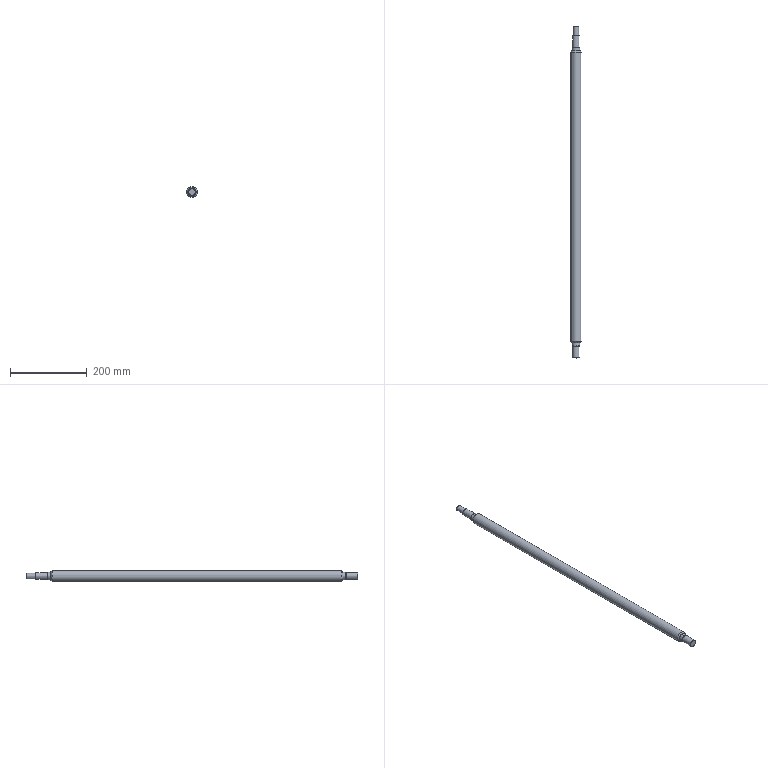Part | NX | features CHAMFER 2, DATUM_CSYS 2, SKETCH 1, SWP104 1, SYMBOLIC_THREAD 1, TRIM BODY 1 | 1 solid | 20 faces | box 28 x 865 x 28 mm | volume 492482 mm3 | plane 7 | cone 7 | cylinder 6 | commonest cylinder face diameters 18 x2 20 x2 14 x1 28 x1
STEP:
#1=CARTESIAN_POINT('',(0.,865.,6.5));
#2=VERTEX_POINT('',#1);
#3=CARTESIAN_POINT('',(0.,865.,0.));
#4=DIRECTION('',(0.,1.,0.));
#5=DIRECTION('',(0.,0.,1.));
#6=AXIS2_PLACEMENT_3D('',#3,#4,#5);
#7=CIRCLE('',#6,6.5);
#8=EDGE_CURVE('',#2,#2,#7,.T.);
#9=ORIENTED_EDGE('',*,*,#8,.T.);
#10=EDGE_LOOP('',(#9));
#11=FACE_BOUND('',#10,.T.);
#12=CARTESIAN_POINT('',(0.,865.,0.));
#13=DIRECTION('',(0.,1.,0.));
#14=DIRECTION('',(0.,0.,1.));
#15=AXIS2_PLACEMENT_3D('',#12,#13,#14);
#16=PLANE('',#15);
#17=ADVANCED_FACE('',(#11),#16,.T.);
#18=CARTESIAN_POINT('',(0.,864.5,7.));
#19=VERTEX_POINT('',#18);
#20=CARTESIAN_POINT('',(0.,864.5,0.));
#21=DIRECTION('',(0.,1.,0.));
#22=DIRECTION('',(0.,0.,1.));
#23=AXIS2_PLACEMENT_3D('',#20,#21,#22);
#24=CIRCLE('',#23,7.);
#25=EDGE_CURVE('',#19,#19,#24,.F.);
#26=ORIENTED_EDGE('',*,*,#25,.T.);
#27=EDGE_LOOP('',(#26));
#28=FACE_BOUND('',#27,.T.);
#29=CARTESIAN_POINT('',(0.,840.,7.));
#30=VERTEX_POINT('',#29);
#31=CARTESIAN_POINT('',(0.,840.,0.));
#32=DIRECTION('',(0.,1.,0.));
#33=DIRECTION('',(0.,0.,1.));
#34=AXIS2_PLACEMENT_3D('',#31,#32,#33);
#35=CIRCLE('',#34,7.);
#36=EDGE_CURVE('',#30,#30,#35,.T.);
#37=ORIENTED_EDGE('',*,*,#36,.T.);
#38=EDGE_LOOP('',(#37));
#39=FACE_BOUND('',#38,.T.);
#40=CARTESIAN_POINT('',(0.,0.,0.));
#41=DIRECTION('',(0.,1.,0.));
#42=DIRECTION('',(0.,0.,1.));
#43=AXIS2_PLACEMENT_3D('',#40,#41,#42);
#44=CYLINDRICAL_SURFACE('',#43,7.);
#45=ADVANCED_FACE('',(#28,#39),#44,.T.);
#46=CARTESIAN_POINT('',(0.,840.,-8.5));
#47=VERTEX_POINT('',#46);
#48=CARTESIAN_POINT('',(0.,840.,0.));
#49=DIRECTION('',(0.,-1.,0.));
#50=DIRECTION('',(0.,0.,-1.));
#51=AXIS2_PLACEMENT_3D('',#48,#49,#50);
#52=CIRCLE('',#51,8.5);
#53=EDGE_CURVE('',#47,#47,#52,.F.);
#54=ORIENTED_EDGE('',*,*,#53,.T.);
#55=EDGE_LOOP('',(#54));
#56=FACE_BOUND('',#55,.T.);
#57=ORIENTED_EDGE('',*,*,#36,.F.);
#58=EDGE_LOOP('',(#57));
#59=FACE_BOUND('',#58,.T.);
#60=CARTESIAN_POINT('',(0.,840.,9.));
#61=DIRECTION('',(0.,-1.,0.));
#62=DIRECTION('',(0.,0.,-1.));
#63=AXIS2_PLACEMENT_3D('',#60,#61,#62);
#64=PLANE('',#63);
#65=ADVANCED_FACE('',(#56,#59),#64,.F.);
#66=CARTESIAN_POINT('',(0.,839.5,-9.));
#67=VERTEX_POINT('',#66);
#68=CARTESIAN_POINT('',(0.,839.5,0.));
#69=DIRECTION('',(0.,-1.,0.));
#70=DIRECTION('',(0.,0.,-1.));
#71=AXIS2_PLACEMENT_3D('',#68,#69,#70);
#72=CIRCLE('',#71,9.);
#73=EDGE_CURVE('',#67,#67,#72,.T.);
#74=ORIENTED_EDGE('',*,*,#73,.T.);
#75=EDGE_LOOP('',(#74));
#76=FACE_BOUND('',#75,.T.);
#77=CARTESIAN_POINT('',(0.,809.,9.));
#78=VERTEX_POINT('',#77);
#79=CARTESIAN_POINT('',(0.,809.,0.));
#80=DIRECTION('',(0.,1.,0.));
#81=DIRECTION('',(0.,0.,1.));
#82=AXIS2_PLACEMENT_3D('',#79,#80,#81);
#83=CIRCLE('',#82,9.);
#84=EDGE_CURVE('',#78,#78,#83,.T.);
#85=ORIENTED_EDGE('',*,*,#84,.T.);
#86=EDGE_LOOP('',(#85));
#87=FACE_BOUND('',#86,.T.);
#88=CARTESIAN_POINT('',(0.,0.,0.));
#89=DIRECTION('',(0.,1.,0.));
#90=DIRECTION('',(0.,0.,1.));
#91=AXIS2_PLACEMENT_3D('',#88,#89,#90);
#92=CYLINDRICAL_SURFACE('',#91,9.);
#93=ADVANCED_FACE('',(#76,#87),#92,.T.);
#94=CARTESIAN_POINT('',(0.,809.,-9.5));
#95=VERTEX_POINT('',#94);
#96=CARTESIAN_POINT('',(0.,809.,0.));
#97=DIRECTION('',(0.,-1.,0.));
#98=DIRECTION('',(0.,0.,-1.));
#99=AXIS2_PLACEMENT_3D('',#96,#97,#98);
#100=CIRCLE('',#99,9.5);
#101=EDGE_CURVE('',#95,#95,#100,.F.);
#102=ORIENTED_EDGE('',*,*,#101,.T.);
#103=EDGE_LOOP('',(#102));
#104=FACE_BOUND('',#103,.T.);
#105=ORIENTED_EDGE('',*,*,#84,.F.);
#106=EDGE_LOOP('',(#105));
#107=FACE_BOUND('',#106,.T.);
#108=CARTESIAN_POINT('',(0.,809.,10.));
#109=DIRECTION('',(0.,-1.,0.));
#110=DIRECTION('',(0.,0.,-1.));
#111=AXIS2_PLACEMENT_3D('',#108,#109,#110);
#112=PLANE('',#111);
#113=ADVANCED_FACE('',(#104,#107),#112,.F.);
#114=CARTESIAN_POINT('',(0.,808.5,-10.));
#115=VERTEX_POINT('',#114);
#116=CARTESIAN_POINT('',(0.,808.5,0.));
#117=DIRECTION('',(0.,-1.,0.));
#118=DIRECTION('',(0.,0.,-1.));
#119=AXIS2_PLACEMENT_3D('',#116,#117,#118);
#120=CIRCLE('',#119,10.);
#121=EDGE_CURVE('',#115,#115,#120,.T.);
#122=ORIENTED_EDGE('',*,*,#121,.T.);
#123=EDGE_LOOP('',(#122));
#124=FACE_BOUND('',#123,.T.);
#125=CARTESIAN_POINT('',(0.,800.,10.));
#126=VERTEX_POINT('',#125);
#127=CARTESIAN_POINT('',(0.,800.,0.));
#128=DIRECTION('',(0.,1.,0.));
#129=DIRECTION('',(0.,0.,1.));
#130=AXIS2_PLACEMENT_3D('',#127,#128,#129);
#131=CIRCLE('',#130,10.);
#132=EDGE_CURVE('',#126,#126,#131,.T.);
#133=ORIENTED_EDGE('',*,*,#132,.T.);
#134=EDGE_LOOP('',(#133));
#135=FACE_BOUND('',#134,.T.);
#136=CARTESIAN_POINT('',(0.,0.,0.));
#137=DIRECTION('',(0.,1.,0.));
#138=DIRECTION('',(0.,0.,1.));
#139=AXIS2_PLACEMENT_3D('',#136,#137,#138);
#140=CYLINDRICAL_SURFACE('',#139,10.);
#141=ADVANCED_FACE('',(#124,#135),#140,.T.);
#142=CARTESIAN_POINT('',(0.,800.,-11.));
#143=VERTEX_POINT('',#142);
#144=CARTESIAN_POINT('',(0.,800.,0.));
#145=DIRECTION('',(0.,-1.,0.));
#146=DIRECTION('',(0.,0.,-1.));
#147=AXIS2_PLACEMENT_3D('',#144,#145,#146);
#148=CIRCLE('',#147,11.);
#149=EDGE_CURVE('',#143,#143,#148,.F.);
#150=ORIENTED_EDGE('',*,*,#149,.T.);
#151=EDGE_LOOP('',(#150));
#152=FACE_BOUND('',#151,.T.);
#153=ORIENTED_EDGE('',*,*,#132,.F.);
#154=EDGE_LOOP('',(#153));
#155=FACE_BOUND('',#154,.T.);
#156=CARTESIAN_POINT('',(0.,800.,14.));
#157=DIRECTION('',(0.,-1.,0.));
#158=DIRECTION('',(0.,0.,-1.));
#159=AXIS2_PLACEMENT_3D('',#156,#157,#158);
#160=PLANE('',#159);
#161=ADVANCED_FACE('',(#152,#155),#160,.F.);
#162=CARTESIAN_POINT('',(0.,43.,14.));
#163=VERTEX_POINT('',#162);
#164=CARTESIAN_POINT('',(0.,43.,0.));
#165=DIRECTION('',(0.,1.,0.));
#166=DIRECTION('',(0.,0.,1.));
#167=AXIS2_PLACEMENT_3D('',#164,#165,#166);
#168=CIRCLE('',#167,14.);
#169=EDGE_CURVE('',#163,#163,#168,.T.);
#170=ORIENTED_EDGE('',*,*,#169,.T.);
#171=EDGE_LOOP('',(#170));
#172=FACE_BOUND('',#171,.T.);
#173=CARTESIAN_POINT('',(0.,797.,-14.));
#174=VERTEX_POINT('',#173);
#175=CARTESIAN_POINT('',(0.,797.,0.));
#176=DIRECTION('',(0.,-1.,0.));
#177=DIRECTION('',(0.,0.,-1.));
#178=AXIS2_PLACEMENT_3D('',#175,#176,#177);
#179=CIRCLE('',#178,14.);
#180=EDGE_CURVE('',#174,#174,#179,.T.);
#181=ORIENTED_EDGE('',*,*,#180,.T.);
#182=EDGE_LOOP('',(#181));
#183=FACE_BOUND('',#182,.T.);
#184=CARTESIAN_POINT('',(0.,0.,0.));
#185=DIRECTION('',(0.,1.,0.));
#186=DIRECTION('',(0.,0.,1.));
#187=AXIS2_PLACEMENT_3D('',#184,#185,#186);
#188=CYLINDRICAL_SURFACE('',#187,14.);
#189=ADVANCED_FACE('',(#172,#183),#188,.T.);
#190=CARTESIAN_POINT('',(0.,40.,11.));
#191=VERTEX_POINT('',#190);
#192=CARTESIAN_POINT('',(0.,40.,0.));
#193=DIRECTION('',(0.,1.,0.));
#194=DIRECTION('',(0.,0.,1.));
#195=AXIS2_PLACEMENT_3D('',#192,#193,#194);
#196=CIRCLE('',#195,11.);
#197=EDGE_CURVE('',#191,#191,#196,.F.);
#198=ORIENTED_EDGE('',*,*,#197,.T.);
#199=EDGE_LOOP('',(#198));
#200=FACE_BOUND('',#199,.T.);
#201=CARTESIAN_POINT('',(0.,40.,10.));
#202=VERTEX_POINT('',#201);
#203=CARTESIAN_POINT('',(0.,40.,0.));
#204=DIRECTION('',(0.,1.,0.));
#205=DIRECTION('',(0.,0.,1.));
#206=AXIS2_PLACEMENT_3D('',#203,#204,#205);
#207=CIRCLE('',#206,10.);
#208=EDGE_CURVE('',#202,#202,#207,.T.);
#209=ORIENTED_EDGE('',*,*,#208,.T.);
#210=EDGE_LOOP('',(#209));
#211=FACE_BOUND('',#210,.T.);
#212=CARTESIAN_POINT('',(0.,40.,10.));
#213=DIRECTION('',(0.,1.,0.));
#214=DIRECTION('',(0.,0.,1.));
#215=AXIS2_PLACEMENT_3D('',#212,#213,#214);
#216=PLANE('',#215);
#217=ADVANCED_FACE('',(#200,#211),#216,.F.);
#218=CARTESIAN_POINT('',(0.,31.5,10.));
#219=VERTEX_POINT('',#218);
#220=CARTESIAN_POINT('',(0.,31.5,0.));
#221=DIRECTION('',(0.,1.,0.));
#222=DIRECTION('',(0.,0.,1.));
#223=AXIS2_PLACEMENT_3D('',#220,#221,#222);
#224=CIRCLE('',#223,10.);
#225=EDGE_CURVE('',#219,#219,#224,.T.);
#226=ORIENTED_EDGE('',*,*,#225,.T.);
#227=EDGE_LOOP('',(#226));
#228=FACE_BOUND('',#227,.T.);
#229=ORIENTED_EDGE('',*,*,#208,.F.);
#230=EDGE_LOOP('',(#229));
#231=FACE_BOUND('',#230,.T.);
#232=CARTESIAN_POINT('',(0.,0.,0.));
#233=DIRECTION('',(0.,1.,0.));
#234=DIRECTION('',(0.,0.,1.));
#235=AXIS2_PLACEMENT_3D('',#232,#233,#234);
#236=CYLINDRICAL_SURFACE('',#235,10.);
#237=ADVANCED_FACE('',(#228,#231),#236,.T.);
#238=CARTESIAN_POINT('',(0.,31.,9.5));
#239=VERTEX_POINT('',#238);
#240=CARTESIAN_POINT('',(0.,31.,0.));
#241=DIRECTION('',(0.,1.,0.));
#242=DIRECTION('',(0.,0.,1.));
#243=AXIS2_PLACEMENT_3D('',#240,#241,#242);
#244=CIRCLE('',#243,9.5);
#245=EDGE_CURVE('',#239,#239,#244,.F.);
#246=ORIENTED_EDGE('',*,*,#245,.T.);
#247=EDGE_LOOP('',(#246));
#248=FACE_BOUND('',#247,.T.);
#249=CARTESIAN_POINT('',(0.,31.,9.));
#250=VERTEX_POINT('',#249);
#251=CARTESIAN_POINT('',(0.,31.,0.));
#252=DIRECTION('',(0.,1.,0.));
#253=DIRECTION('',(0.,0.,1.));
#254=AXIS2_PLACEMENT_3D('',#251,#252,#253);
#255=CIRCLE('',#254,9.);
#256=EDGE_CURVE('',#250,#250,#255,.T.);
#257=ORIENTED_EDGE('',*,*,#256,.T.);
#258=EDGE_LOOP('',(#257));
#259=FACE_BOUND('',#258,.T.);
#260=CARTESIAN_POINT('',(0.,31.,9.));
#261=DIRECTION('',(0.,1.,0.));
#262=DIRECTION('',(0.,0.,1.));
#263=AXIS2_PLACEMENT_3D('',#260,#261,#262);
#264=PLANE('',#263);
#265=ADVANCED_FACE('',(#248,#259),#264,.F.);
#266=CARTESIAN_POINT('',(0.,0.5,9.));
#267=VERTEX_POINT('',#266);
#268=CARTESIAN_POINT('',(0.,0.5,0.));
#269=DIRECTION('',(0.,1.,0.));
#270=DIRECTION('',(0.,0.,1.));
#271=AXIS2_PLACEMENT_3D('',#268,#269,#270);
#272=CIRCLE('',#271,9.);
#273=EDGE_CURVE('',#267,#267,#272,.T.);
#274=ORIENTED_EDGE('',*,*,#273,.T.);
#275=EDGE_LOOP('',(#274));
#276=FACE_BOUND('',#275,.T.);
#277=ORIENTED_EDGE('',*,*,#256,.F.);
#278=EDGE_LOOP('',(#277));
#279=FACE_BOUND('',#278,.T.);
#280=CARTESIAN_POINT('',(0.,0.,0.));
#281=DIRECTION('',(0.,1.,0.));
#282=DIRECTION('',(0.,0.,1.));
#283=AXIS2_PLACEMENT_3D('',#280,#281,#282);
#284=CYLINDRICAL_SURFACE('',#283,9.);
#285=ADVANCED_FACE('',(#276,#279),#284,.T.);
#286=CARTESIAN_POINT('',(0.,0.,8.5));
#287=VERTEX_POINT('',#286);
#288=CARTESIAN_POINT('',(0.,0.,0.));
#289=DIRECTION('',(0.,1.,0.));
#290=DIRECTION('',(0.,0.,1.));
#291=AXIS2_PLACEMENT_3D('',#288,#289,#290);
#292=CIRCLE('',#291,8.5);
#293=EDGE_CURVE('',#287,#287,#292,.F.);
#294=ORIENTED_EDGE('',*,*,#293,.T.);
#295=EDGE_LOOP('',(#294));
#296=FACE_BOUND('',#295,.T.);
#297=CARTESIAN_POINT('',(0.,0.,7.));
#298=DIRECTION('',(0.,1.,0.));
#299=DIRECTION('',(0.,0.,1.));
#300=AXIS2_PLACEMENT_3D('',#297,#298,#299);
#301=PLANE('',#300);
#302=ADVANCED_FACE('',(#296),#301,.F.);
#303=ORIENTED_EDGE('',*,*,#197,.F.);
#304=EDGE_LOOP('',(#303));
#305=FACE_BOUND('',#304,.T.);
#306=ORIENTED_EDGE('',*,*,#169,.F.);
#307=EDGE_LOOP('',(#306));
#308=FACE_BOUND('',#307,.T.);
#309=CARTESIAN_POINT('',(0.,43.,0.));
#310=DIRECTION('',(0.,1.,0.));
#311=DIRECTION('',(0.,0.,1.));
#312=AXIS2_PLACEMENT_3D('',#309,#310,#311);
#313=CONICAL_SURFACE('',#312,14.,0.7854);
#314=ADVANCED_FACE('',(#305,#308),#313,.T.);
#315=ORIENTED_EDGE('',*,*,#180,.F.);
#316=EDGE_LOOP('',(#315));
#317=FACE_BOUND('',#316,.T.);
#318=ORIENTED_EDGE('',*,*,#149,.F.);
#319=EDGE_LOOP('',(#318));
#320=FACE_BOUND('',#319,.T.);
#321=CARTESIAN_POINT('',(0.,800.,0.));
#322=DIRECTION('',(0.,-1.,0.));
#323=DIRECTION('',(0.,0.,-1.));
#324=AXIS2_PLACEMENT_3D('',#321,#322,#323);
#325=CONICAL_SURFACE('',#324,11.,0.7854);
#326=ADVANCED_FACE('',(#317,#320),#325,.T.);
#327=ORIENTED_EDGE('',*,*,#73,.F.);
#328=EDGE_LOOP('',(#327));
#329=FACE_BOUND('',#328,.T.);
#330=ORIENTED_EDGE('',*,*,#53,.F.);
#331=EDGE_LOOP('',(#330));
#332=FACE_BOUND('',#331,.T.);
#333=CARTESIAN_POINT('',(0.,840.,0.));
#334=DIRECTION('',(0.,-1.,0.));
#335=DIRECTION('',(0.,0.,-1.));
#336=AXIS2_PLACEMENT_3D('',#333,#334,#335);
#337=CONICAL_SURFACE('',#336,8.5,0.7854);
#338=ADVANCED_FACE('',(#329,#332),#337,.T.);
#339=ORIENTED_EDGE('',*,*,#121,.F.);
#340=EDGE_LOOP('',(#339));
#341=FACE_BOUND('',#340,.T.);
#342=ORIENTED_EDGE('',*,*,#101,.F.);
#343=EDGE_LOOP('',(#342));
#344=FACE_BOUND('',#343,.T.);
#345=CARTESIAN_POINT('',(0.,809.,0.));
#346=DIRECTION('',(0.,-1.,0.));
#347=DIRECTION('',(0.,0.,-1.));
#348=AXIS2_PLACEMENT_3D('',#345,#346,#347);
#349=CONICAL_SURFACE('',#348,9.5,0.7854);
#350=ADVANCED_FACE('',(#341,#344),#349,.T.);
#351=ORIENTED_EDGE('',*,*,#25,.F.);
#352=EDGE_LOOP('',(#351));
#353=FACE_BOUND('',#352,.T.);
#354=ORIENTED_EDGE('',*,*,#8,.F.);
#355=EDGE_LOOP('',(#354));
#356=FACE_BOUND('',#355,.T.);
#357=CARTESIAN_POINT('',(0.,865.,0.));
#358=DIRECTION('',(0.,-1.,0.));
#359=DIRECTION('',(0.,0.,-1.));
#360=AXIS2_PLACEMENT_3D('',#357,#358,#359);
#361=CONICAL_SURFACE('',#360,6.5,0.7854);
#362=ADVANCED_FACE('',(#353,#356),#361,.T.);
#363=ORIENTED_EDGE('',*,*,#293,.F.);
#364=EDGE_LOOP('',(#363));
#365=FACE_BOUND('',#364,.T.);
#366=ORIENTED_EDGE('',*,*,#273,.F.);
#367=EDGE_LOOP('',(#366));
#368=FACE_BOUND('',#367,.T.);
#369=CARTESIAN_POINT('',(0.,0.5,0.));
#370=DIRECTION('',(0.,1.,0.));
#371=DIRECTION('',(0.,0.,1.));
#372=AXIS2_PLACEMENT_3D('',#369,#370,#371);
#373=CONICAL_SURFACE('',#372,9.,0.7854);
#374=ADVANCED_FACE('',(#365,#368),#373,.T.);
#375=ORIENTED_EDGE('',*,*,#245,.F.);
#376=EDGE_LOOP('',(#375));
#377=FACE_BOUND('',#376,.T.);
#378=ORIENTED_EDGE('',*,*,#225,.F.);
#379=EDGE_LOOP('',(#378));
#380=FACE_BOUND('',#379,.T.);
#381=CARTESIAN_POINT('',(0.,31.5,0.));
#382=DIRECTION('',(0.,1.,0.));
#383=DIRECTION('',(0.,0.,1.));
#384=AXIS2_PLACEMENT_3D('',#381,#382,#383);
#385=CONICAL_SURFACE('',#384,10.,0.7854);
#386=ADVANCED_FACE('',(#377,#380),#385,.T.);
#387=CLOSED_SHELL('',(#17,#45,#65,#93,#113,#141,#161,#189,#217,#237,#265,#285,#302,#314,#326,#338,#350,#362,#374,#386));
#388=MANIFOLD_SOLID_BREP('',#387);
#389=(LENGTH_UNIT()NAMED_UNIT(*)SI_UNIT(.MILLI.,.METRE.));
#390=UNCERTAINTY_MEASURE_WITH_UNIT(LENGTH_MEASURE(0.00001),#389,'','');
#391=(NAMED_UNIT(*)PLANE_ANGLE_UNIT()SI_UNIT($,.RADIAN.));
#392=(NAMED_UNIT(*)SI_UNIT($,.STERADIAN.)SOLID_ANGLE_UNIT());
#393=(GEOMETRIC_REPRESENTATION_CONTEXT(3)GLOBAL_UNCERTAINTY_ASSIGNED_CONTEXT((#390))GLOBAL_UNIT_ASSIGNED_CONTEXT((#389,#391,#392))REPRESENTATION_CONTEXT('',''));
#394=ADVANCED_BREP_SHAPE_REPRESENTATION('',(#388),#393);